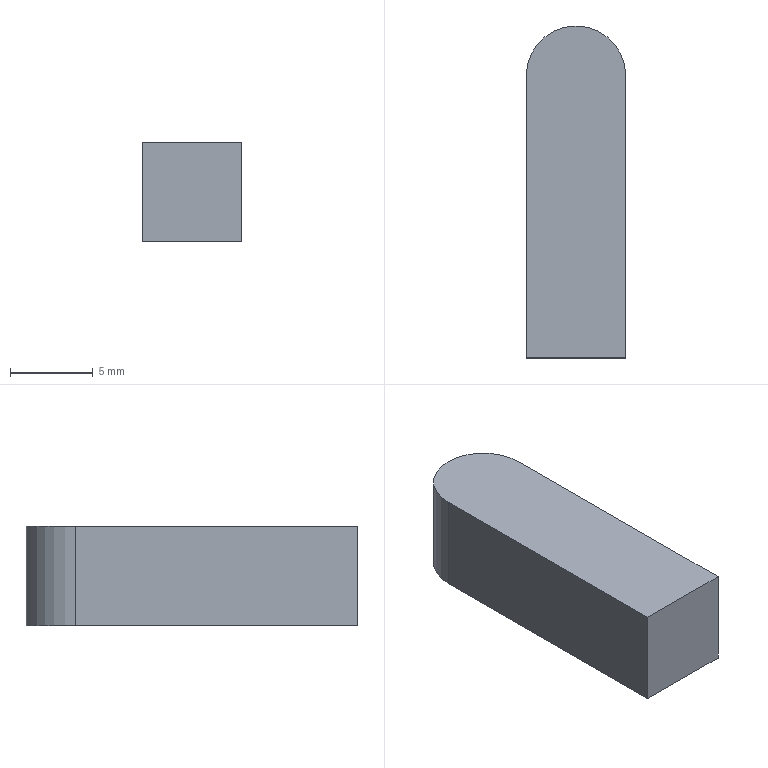Part | NX | features DATUM_CSYS 2, EXTRUDE 1, FACE_BLEND 1, SKETCH 1 | 1 solid | 6 faces | box 6 x 20 x 6 mm | volume 696.823 mm3 | plane 5 | cylinder 1 | commonest cylinder face diameters 6 x1
STEP:
#1=CARTESIAN_POINT('',(0.,17.,0.));
#2=VERTEX_POINT('',#1);
#3=CARTESIAN_POINT('',(0.,17.,6.));
#4=VERTEX_POINT('',#3);
#5=CARTESIAN_POINT('',(0.,17.,6.));
#6=DIRECTION('',(0.,0.,1.));
#7=VECTOR('',#6,1000.);
#8=LINE('',#5,#7);
#9=EDGE_CURVE('',#2,#4,#8,.T.);
#10=ORIENTED_EDGE('',*,*,#9,.F.);
#11=CARTESIAN_POINT('',(-6.,17.,0.));
#12=VERTEX_POINT('',#11);
#13=CARTESIAN_POINT('',(-3.,17.,0.));
#14=DIRECTION('',(0.,0.,1.));
#15=DIRECTION('',(1.,0.,0.));
#16=AXIS2_PLACEMENT_3D('',#13,#14,#15);
#17=CIRCLE('',#16,3.);
#18=EDGE_CURVE('',#12,#2,#17,.F.);
#19=ORIENTED_EDGE('',*,*,#18,.F.);
#20=CARTESIAN_POINT('',(-6.,17.,6.));
#21=VERTEX_POINT('',#20);
#22=CARTESIAN_POINT('',(-6.,17.,6.));
#23=DIRECTION('',(0.,0.,1.));
#24=VECTOR('',#23,1000.);
#25=LINE('',#22,#24);
#26=EDGE_CURVE('',#21,#12,#25,.F.);
#27=ORIENTED_EDGE('',*,*,#26,.F.);
#28=CARTESIAN_POINT('',(-3.,17.,6.));
#29=DIRECTION('',(0.,0.,1.));
#30=DIRECTION('',(1.,0.,0.));
#31=AXIS2_PLACEMENT_3D('',#28,#29,#30);
#32=CIRCLE('',#31,3.);
#33=EDGE_CURVE('',#4,#21,#32,.T.);
#34=ORIENTED_EDGE('',*,*,#33,.F.);
#35=EDGE_LOOP('',(#10,#19,#27,#34));
#36=FACE_BOUND('',#35,.T.);
#37=CARTESIAN_POINT('',(-3.,17.,0.));
#38=DIRECTION('',(0.,0.,1.));
#39=DIRECTION('',(1.,0.,0.));
#40=AXIS2_PLACEMENT_3D('',#37,#38,#39);
#41=CYLINDRICAL_SURFACE('',#40,3.);
#42=ADVANCED_FACE('',(#36),#41,.T.);
#43=CARTESIAN_POINT('',(-6.,0.,6.));
#44=VERTEX_POINT('',#43);
#45=CARTESIAN_POINT('',(-6.,20.,6.));
#46=DIRECTION('',(0.,-1.,0.));
#47=VECTOR('',#46,1000.);
#48=LINE('',#45,#47);
#49=EDGE_CURVE('',#21,#44,#48,.T.);
#50=ORIENTED_EDGE('',*,*,#49,.F.);
#51=ORIENTED_EDGE('',*,*,#26,.T.);
#52=CARTESIAN_POINT('',(-6.,0.,0.));
#53=VERTEX_POINT('',#52);
#54=CARTESIAN_POINT('',(-6.,20.,0.));
#55=DIRECTION('',(0.,-1.,0.));
#56=VECTOR('',#55,1000.);
#57=LINE('',#54,#56);
#58=EDGE_CURVE('',#12,#53,#57,.T.);
#59=ORIENTED_EDGE('',*,*,#58,.T.);
#60=CARTESIAN_POINT('',(-6.,0.,6.));
#61=DIRECTION('',(0.,0.,-1.));
#62=VECTOR('',#61,1000.);
#63=LINE('',#60,#62);
#64=EDGE_CURVE('',#44,#53,#63,.T.);
#65=ORIENTED_EDGE('',*,*,#64,.F.);
#66=EDGE_LOOP('',(#50,#51,#59,#65));
#67=FACE_BOUND('',#66,.T.);
#68=CARTESIAN_POINT('',(-6.,20.,6.));
#69=DIRECTION('',(1.,0.,0.));
#70=DIRECTION('',(0.,1.,0.));
#71=AXIS2_PLACEMENT_3D('',#68,#69,#70);
#72=PLANE('',#71);
#73=ADVANCED_FACE('',(#67),#72,.F.);
#74=CARTESIAN_POINT('',(0.,0.,0.));
#75=VERTEX_POINT('',#74);
#76=CARTESIAN_POINT('',(-6.,0.,0.));
#77=DIRECTION('',(1.,0.,0.));
#78=VECTOR('',#77,1000.);
#79=LINE('',#76,#78);
#80=EDGE_CURVE('',#53,#75,#79,.T.);
#81=ORIENTED_EDGE('',*,*,#80,.T.);
#82=CARTESIAN_POINT('',(0.,0.,6.));
#83=VERTEX_POINT('',#82);
#84=CARTESIAN_POINT('',(0.,0.,6.));
#85=DIRECTION('',(0.,0.,-1.));
#86=VECTOR('',#85,1000.);
#87=LINE('',#84,#86);
#88=EDGE_CURVE('',#83,#75,#87,.T.);
#89=ORIENTED_EDGE('',*,*,#88,.F.);
#90=CARTESIAN_POINT('',(-6.,0.,6.));
#91=DIRECTION('',(1.,0.,0.));
#92=VECTOR('',#91,1000.);
#93=LINE('',#90,#92);
#94=EDGE_CURVE('',#44,#83,#93,.T.);
#95=ORIENTED_EDGE('',*,*,#94,.F.);
#96=ORIENTED_EDGE('',*,*,#64,.T.);
#97=EDGE_LOOP('',(#81,#89,#95,#96));
#98=FACE_BOUND('',#97,.T.);
#99=CARTESIAN_POINT('',(-6.,0.,6.));
#100=DIRECTION('',(0.,1.,0.));
#101=DIRECTION('',(-1.,0.,0.));
#102=AXIS2_PLACEMENT_3D('',#99,#100,#101);
#103=PLANE('',#102);
#104=ADVANCED_FACE('',(#98),#103,.F.);
#105=CARTESIAN_POINT('',(0.,0.,0.));
#106=DIRECTION('',(0.,1.,0.));
#107=VECTOR('',#106,1000.);
#108=LINE('',#105,#107);
#109=EDGE_CURVE('',#75,#2,#108,.T.);
#110=ORIENTED_EDGE('',*,*,#109,.T.);
#111=ORIENTED_EDGE('',*,*,#9,.T.);
#112=CARTESIAN_POINT('',(0.,0.,6.));
#113=DIRECTION('',(0.,1.,0.));
#114=VECTOR('',#113,1000.);
#115=LINE('',#112,#114);
#116=EDGE_CURVE('',#83,#4,#115,.T.);
#117=ORIENTED_EDGE('',*,*,#116,.F.);
#118=ORIENTED_EDGE('',*,*,#88,.T.);
#119=EDGE_LOOP('',(#110,#111,#117,#118));
#120=FACE_BOUND('',#119,.T.);
#121=CARTESIAN_POINT('',(0.,0.,6.));
#122=DIRECTION('',(-1.,0.,0.));
#123=DIRECTION('',(0.,-1.,0.));
#124=AXIS2_PLACEMENT_3D('',#121,#122,#123);
#125=PLANE('',#124);
#126=ADVANCED_FACE('',(#120),#125,.F.);
#127=ORIENTED_EDGE('',*,*,#116,.T.);
#128=ORIENTED_EDGE('',*,*,#33,.T.);
#129=ORIENTED_EDGE('',*,*,#49,.T.);
#130=ORIENTED_EDGE('',*,*,#94,.T.);
#131=EDGE_LOOP('',(#127,#128,#129,#130));
#132=FACE_BOUND('',#131,.T.);
#133=CARTESIAN_POINT('',(0.,0.,6.));
#134=DIRECTION('',(0.,0.,1.));
#135=DIRECTION('',(1.,0.,0.));
#136=AXIS2_PLACEMENT_3D('',#133,#134,#135);
#137=PLANE('',#136);
#138=ADVANCED_FACE('',(#132),#137,.T.);
#139=ORIENTED_EDGE('',*,*,#58,.F.);
#140=ORIENTED_EDGE('',*,*,#18,.T.);
#141=ORIENTED_EDGE('',*,*,#109,.F.);
#142=ORIENTED_EDGE('',*,*,#80,.F.);
#143=EDGE_LOOP('',(#139,#140,#141,#142));
#144=FACE_BOUND('',#143,.T.);
#145=CARTESIAN_POINT('',(0.,0.,0.));
#146=DIRECTION('',(0.,0.,1.));
#147=DIRECTION('',(1.,0.,0.));
#148=AXIS2_PLACEMENT_3D('',#145,#146,#147);
#149=PLANE('',#148);
#150=ADVANCED_FACE('',(#144),#149,.F.);
#151=CLOSED_SHELL('',(#42,#73,#104,#126,#138,#150));
#152=MANIFOLD_SOLID_BREP('',#151);
#153=(LENGTH_UNIT()NAMED_UNIT(*)SI_UNIT(.MILLI.,.METRE.));
#154=UNCERTAINTY_MEASURE_WITH_UNIT(LENGTH_MEASURE(0.00001),#153,'','');
#155=(NAMED_UNIT(*)PLANE_ANGLE_UNIT()SI_UNIT($,.RADIAN.));
#156=(NAMED_UNIT(*)SI_UNIT($,.STERADIAN.)SOLID_ANGLE_UNIT());
#157=(GEOMETRIC_REPRESENTATION_CONTEXT(3)GLOBAL_UNCERTAINTY_ASSIGNED_CONTEXT((#154))GLOBAL_UNIT_ASSIGNED_CONTEXT((#153,#155,#156))REPRESENTATION_CONTEXT('',''));
#158=ADVANCED_BREP_SHAPE_REPRESENTATION('',(#152),#157);